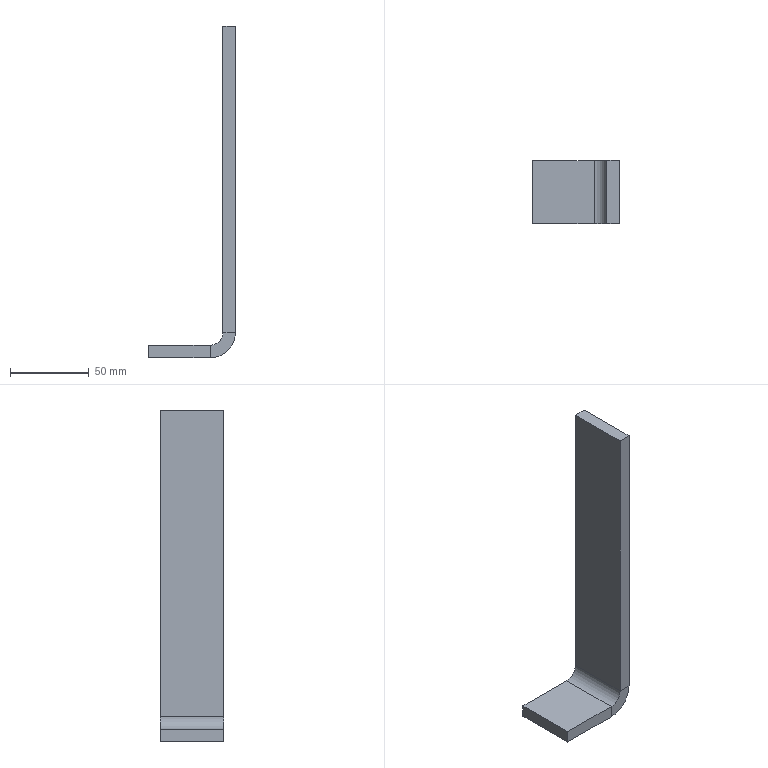Part | SolidWorks | features FlatPattern 1, SM3dBend 1, SMBaseFlange 1, SheetMetal 1 | 1 solid | 14 faces | box 55 x 40 x 210.02 mm | volume 80598 mm3 | plane 12 | cylinder 2 | commonest cylinder face diameters 16 x1 32 x1
STEP:
#1=CARTESIAN_POINT('',(-70.935,-20.,8.));
#2=VERTEX_POINT('',#1);
#3=CARTESIAN_POINT('',(-70.935,-20.,202.02));
#4=VERTEX_POINT('',#3);
#5=CARTESIAN_POINT('',(-70.935,-20.,-49.85));
#6=DIRECTION('',(0.,0.,1.));
#7=VECTOR('',#6,1000.);
#8=LINE('',#5,#7);
#9=EDGE_CURVE('',#2,#4,#8,.T.);
#10=ORIENTED_EDGE('',*,*,#9,.F.);
#11=CARTESIAN_POINT('',(-70.935,20.,8.));
#12=VERTEX_POINT('',#11);
#13=CARTESIAN_POINT('',(-70.935,0.,8.));
#14=DIRECTION('',(0.,1.,0.));
#15=VECTOR('',#14,1000.);
#16=LINE('',#13,#15);
#17=EDGE_CURVE('',#2,#12,#16,.T.);
#18=ORIENTED_EDGE('',*,*,#17,.T.);
#19=CARTESIAN_POINT('',(-70.935,20.,202.02));
#20=VERTEX_POINT('',#19);
#21=CARTESIAN_POINT('',(-70.935,20.,-49.85));
#22=DIRECTION('',(0.,0.,-1.));
#23=VECTOR('',#22,1000.);
#24=LINE('',#21,#23);
#25=EDGE_CURVE('',#20,#12,#24,.T.);
#26=ORIENTED_EDGE('',*,*,#25,.F.);
#27=CARTESIAN_POINT('',(-70.935,20.,202.02));
#28=DIRECTION('',(0.,1.,0.));
#29=VECTOR('',#28,1000.);
#30=LINE('',#27,#29);
#31=EDGE_CURVE('',#4,#20,#30,.T.);
#32=ORIENTED_EDGE('',*,*,#31,.F.);
#33=EDGE_LOOP('',(#10,#18,#26,#32));
#34=FACE_OUTER_BOUND('',#33,.T.);
#35=CARTESIAN_POINT('',(-70.935,0.,76.085));
#36=DIRECTION('',(-1.,0.,0.));
#37=DIRECTION('',(0.,0.,1.));
#38=AXIS2_PLACEMENT_3D('',#35,#36,#37);
#39=PLANE('',#38);
#40=ADVANCED_FACE('',(#34),#39,.F.);
#41=CARTESIAN_POINT('',(-78.935,-20.,202.02));
#42=VERTEX_POINT('',#41);
#43=CARTESIAN_POINT('',(-78.935,20.,202.02));
#44=VERTEX_POINT('',#43);
#45=CARTESIAN_POINT('',(-78.935,20.,202.02));
#46=DIRECTION('',(0.,1.,0.));
#47=VECTOR('',#46,1000.);
#48=LINE('',#45,#47);
#49=EDGE_CURVE('',#42,#44,#48,.T.);
#50=ORIENTED_EDGE('',*,*,#49,.F.);
#51=CARTESIAN_POINT('',(-70.935,-20.,202.02));
#52=DIRECTION('',(-1.,0.,0.));
#53=VECTOR('',#52,1000.);
#54=LINE('',#51,#53);
#55=EDGE_CURVE('',#4,#42,#54,.T.);
#56=ORIENTED_EDGE('',*,*,#55,.F.);
#57=ORIENTED_EDGE('',*,*,#31,.T.);
#58=CARTESIAN_POINT('',(-70.935,20.,202.02));
#59=DIRECTION('',(-1.,0.,0.));
#60=VECTOR('',#59,1000.);
#61=LINE('',#58,#60);
#62=EDGE_CURVE('',#20,#44,#61,.T.);
#63=ORIENTED_EDGE('',*,*,#62,.T.);
#64=EDGE_LOOP('',(#50,#56,#57,#63));
#65=FACE_OUTER_BOUND('',#64,.T.);
#66=CARTESIAN_POINT('',(-70.935,20.,202.02));
#67=DIRECTION('',(0.,0.,1.));
#68=DIRECTION('',(1.,0.,0.));
#69=AXIS2_PLACEMENT_3D('',#66,#67,#68);
#70=PLANE('',#69);
#71=ADVANCED_FACE('',(#65),#70,.T.);
#72=CARTESIAN_POINT('',(-78.935,-20.,8.));
#73=VERTEX_POINT('',#72);
#74=CARTESIAN_POINT('',(-70.935,-20.,8.));
#75=DIRECTION('',(-1.,0.,0.));
#76=VECTOR('',#75,1000.);
#77=LINE('',#74,#76);
#78=EDGE_CURVE('',#2,#73,#77,.T.);
#79=ORIENTED_EDGE('',*,*,#78,.F.);
#80=ORIENTED_EDGE('',*,*,#9,.T.);
#81=ORIENTED_EDGE('',*,*,#55,.T.);
#82=CARTESIAN_POINT('',(-78.935,-20.,-49.85));
#83=DIRECTION('',(0.,0.,1.));
#84=VECTOR('',#83,1000.);
#85=LINE('',#82,#84);
#86=EDGE_CURVE('',#73,#42,#85,.T.);
#87=ORIENTED_EDGE('',*,*,#86,.F.);
#88=EDGE_LOOP('',(#79,#80,#81,#87));
#89=FACE_OUTER_BOUND('',#88,.T.);
#90=CARTESIAN_POINT('',(-70.935,-20.,-49.85));
#91=DIRECTION('',(0.,-1.,0.));
#92=DIRECTION('',(1.,0.,0.));
#93=AXIS2_PLACEMENT_3D('',#90,#91,#92);
#94=PLANE('',#93);
#95=ADVANCED_FACE('',(#89),#94,.T.);
#96=CARTESIAN_POINT('',(-78.935,20.,8.));
#97=VERTEX_POINT('',#96);
#98=CARTESIAN_POINT('',(-70.935,20.,8.));
#99=DIRECTION('',(1.,0.,0.));
#100=VECTOR('',#99,1000.);
#101=LINE('',#98,#100);
#102=EDGE_CURVE('',#97,#12,#101,.T.);
#103=ORIENTED_EDGE('',*,*,#102,.F.);
#104=CARTESIAN_POINT('',(-78.935,20.,-49.85));
#105=DIRECTION('',(0.,0.,-1.));
#106=VECTOR('',#105,1000.);
#107=LINE('',#104,#106);
#108=EDGE_CURVE('',#44,#97,#107,.T.);
#109=ORIENTED_EDGE('',*,*,#108,.F.);
#110=ORIENTED_EDGE('',*,*,#62,.F.);
#111=ORIENTED_EDGE('',*,*,#25,.T.);
#112=EDGE_LOOP('',(#103,#109,#110,#111));
#113=FACE_OUTER_BOUND('',#112,.T.);
#114=CARTESIAN_POINT('',(-70.935,20.,-49.85));
#115=DIRECTION('',(0.,1.,0.));
#116=DIRECTION('',(-1.,0.,0.));
#117=AXIS2_PLACEMENT_3D('',#114,#115,#116);
#118=PLANE('',#117);
#119=ADVANCED_FACE('',(#113),#118,.T.);
#120=CARTESIAN_POINT('',(-78.935,0.,8.));
#121=DIRECTION('',(0.,1.,0.));
#122=VECTOR('',#121,1000.);
#123=LINE('',#120,#122);
#124=EDGE_CURVE('',#73,#97,#123,.T.);
#125=ORIENTED_EDGE('',*,*,#124,.F.);
#126=ORIENTED_EDGE('',*,*,#86,.T.);
#127=ORIENTED_EDGE('',*,*,#49,.T.);
#128=ORIENTED_EDGE('',*,*,#108,.T.);
#129=EDGE_LOOP('',(#125,#126,#127,#128));
#130=FACE_OUTER_BOUND('',#129,.T.);
#131=CARTESIAN_POINT('',(-78.935,0.,76.085));
#132=DIRECTION('',(-1.,0.,0.));
#133=DIRECTION('',(0.,0.,1.));
#134=AXIS2_PLACEMENT_3D('',#131,#132,#133);
#135=PLANE('',#134);
#136=ADVANCED_FACE('',(#130),#135,.T.);
#137=CARTESIAN_POINT('',(-125.935,20.,0.));
#138=VERTEX_POINT('',#137);
#139=CARTESIAN_POINT('',(-125.935,-20.,0.));
#140=VERTEX_POINT('',#139);
#141=CARTESIAN_POINT('',(-125.935,20.,0.));
#142=DIRECTION('',(0.,-1.,0.));
#143=VECTOR('',#142,1000.);
#144=LINE('',#141,#143);
#145=EDGE_CURVE('',#138,#140,#144,.T.);
#146=ORIENTED_EDGE('',*,*,#145,.F.);
#147=CARTESIAN_POINT('',(-125.935,20.,-8.));
#148=VERTEX_POINT('',#147);
#149=CARTESIAN_POINT('',(-125.935,20.,-8.));
#150=DIRECTION('',(0.,0.,1.));
#151=VECTOR('',#150,1000.);
#152=LINE('',#149,#151);
#153=EDGE_CURVE('',#148,#138,#152,.T.);
#154=ORIENTED_EDGE('',*,*,#153,.F.);
#155=CARTESIAN_POINT('',(-125.935,-20.,-8.));
#156=VERTEX_POINT('',#155);
#157=CARTESIAN_POINT('',(-125.935,20.,-8.));
#158=DIRECTION('',(0.,-1.,0.));
#159=VECTOR('',#158,1000.);
#160=LINE('',#157,#159);
#161=EDGE_CURVE('',#148,#156,#160,.T.);
#162=ORIENTED_EDGE('',*,*,#161,.T.);
#163=CARTESIAN_POINT('',(-125.935,-20.,-8.));
#164=DIRECTION('',(0.,0.,1.));
#165=VECTOR('',#164,1000.);
#166=LINE('',#163,#165);
#167=EDGE_CURVE('',#156,#140,#166,.T.);
#168=ORIENTED_EDGE('',*,*,#167,.T.);
#169=EDGE_LOOP('',(#146,#154,#162,#168));
#170=FACE_OUTER_BOUND('',#169,.T.);
#171=CARTESIAN_POINT('',(-125.935,20.,-8.));
#172=DIRECTION('',(-1.,0.,0.));
#173=DIRECTION('',(0.,0.,1.));
#174=AXIS2_PLACEMENT_3D('',#171,#172,#173);
#175=PLANE('',#174);
#176=ADVANCED_FACE('',(#170),#175,.T.);
#177=CARTESIAN_POINT('',(-86.935,-20.,-8.));
#178=VERTEX_POINT('',#177);
#179=CARTESIAN_POINT('',(-86.935,20.,-8.));
#180=VERTEX_POINT('',#179);
#181=CARTESIAN_POINT('',(-86.935,0.,-8.));
#182=DIRECTION('',(0.,1.,0.));
#183=VECTOR('',#182,1000.);
#184=LINE('',#181,#183);
#185=EDGE_CURVE('',#178,#180,#184,.T.);
#186=ORIENTED_EDGE('',*,*,#185,.F.);
#187=CARTESIAN_POINT('',(-125.935,-20.,-8.));
#188=DIRECTION('',(1.,0.,0.));
#189=VECTOR('',#188,1000.);
#190=LINE('',#187,#189);
#191=EDGE_CURVE('',#156,#178,#190,.T.);
#192=ORIENTED_EDGE('',*,*,#191,.F.);
#193=ORIENTED_EDGE('',*,*,#161,.F.);
#194=CARTESIAN_POINT('',(-125.935,20.,-8.));
#195=DIRECTION('',(-1.,0.,0.));
#196=VECTOR('',#195,1000.);
#197=LINE('',#194,#196);
#198=EDGE_CURVE('',#180,#148,#197,.T.);
#199=ORIENTED_EDGE('',*,*,#198,.F.);
#200=EDGE_LOOP('',(#186,#192,#193,#199));
#201=FACE_OUTER_BOUND('',#200,.T.);
#202=CARTESIAN_POINT('',(0.,0.,-8.));
#203=DIRECTION('',(0.,0.,1.));
#204=DIRECTION('',(1.,0.,0.));
#205=AXIS2_PLACEMENT_3D('',#202,#203,#204);
#206=PLANE('',#205);
#207=ADVANCED_FACE('',(#201),#206,.F.);
#208=ORIENTED_EDGE('',*,*,#191,.T.);
#209=CARTESIAN_POINT('',(-86.935,-20.,0.));
#210=VERTEX_POINT('',#209);
#211=CARTESIAN_POINT('',(-86.935,-20.,-8.));
#212=DIRECTION('',(0.,0.,1.));
#213=VECTOR('',#212,1000.);
#214=LINE('',#211,#213);
#215=EDGE_CURVE('',#178,#210,#214,.T.);
#216=ORIENTED_EDGE('',*,*,#215,.T.);
#217=CARTESIAN_POINT('',(-125.935,-20.,0.));
#218=DIRECTION('',(1.,0.,0.));
#219=VECTOR('',#218,1000.);
#220=LINE('',#217,#219);
#221=EDGE_CURVE('',#140,#210,#220,.T.);
#222=ORIENTED_EDGE('',*,*,#221,.F.);
#223=ORIENTED_EDGE('',*,*,#167,.F.);
#224=EDGE_LOOP('',(#208,#216,#222,#223));
#225=FACE_OUTER_BOUND('',#224,.T.);
#226=CARTESIAN_POINT('',(-125.935,-20.,-8.));
#227=DIRECTION('',(0.,-1.,0.));
#228=DIRECTION('',(0.,0.,-1.));
#229=AXIS2_PLACEMENT_3D('',#226,#227,#228);
#230=PLANE('',#229);
#231=ADVANCED_FACE('',(#225),#230,.T.);
#232=ORIENTED_EDGE('',*,*,#221,.T.);
#233=CARTESIAN_POINT('',(-86.935,20.,0.));
#234=VERTEX_POINT('',#233);
#235=CARTESIAN_POINT('',(-86.935,0.,0.));
#236=DIRECTION('',(0.,1.,0.));
#237=VECTOR('',#236,1000.);
#238=LINE('',#235,#237);
#239=EDGE_CURVE('',#210,#234,#238,.T.);
#240=ORIENTED_EDGE('',*,*,#239,.T.);
#241=CARTESIAN_POINT('',(-125.935,20.,0.));
#242=DIRECTION('',(-1.,0.,0.));
#243=VECTOR('',#242,1000.);
#244=LINE('',#241,#243);
#245=EDGE_CURVE('',#234,#138,#244,.T.);
#246=ORIENTED_EDGE('',*,*,#245,.T.);
#247=ORIENTED_EDGE('',*,*,#145,.T.);
#248=EDGE_LOOP('',(#232,#240,#246,#247));
#249=FACE_OUTER_BOUND('',#248,.T.);
#250=CARTESIAN_POINT('',(0.,0.,0.));
#251=DIRECTION('',(0.,0.,1.));
#252=DIRECTION('',(1.,0.,0.));
#253=AXIS2_PLACEMENT_3D('',#250,#251,#252);
#254=PLANE('',#253);
#255=ADVANCED_FACE('',(#249),#254,.T.);
#256=ORIENTED_EDGE('',*,*,#245,.F.);
#257=CARTESIAN_POINT('',(-86.935,20.,-8.));
#258=DIRECTION('',(0.,0.,-1.));
#259=VECTOR('',#258,1000.);
#260=LINE('',#257,#259);
#261=EDGE_CURVE('',#234,#180,#260,.T.);
#262=ORIENTED_EDGE('',*,*,#261,.T.);
#263=ORIENTED_EDGE('',*,*,#198,.T.);
#264=ORIENTED_EDGE('',*,*,#153,.T.);
#265=EDGE_LOOP('',(#256,#262,#263,#264));
#266=FACE_OUTER_BOUND('',#265,.T.);
#267=CARTESIAN_POINT('',(-125.935,20.,-8.));
#268=DIRECTION('',(0.,1.,0.));
#269=DIRECTION('',(0.,0.,1.));
#270=AXIS2_PLACEMENT_3D('',#267,#268,#269);
#271=PLANE('',#270);
#272=ADVANCED_FACE('',(#266),#271,.T.);
#273=ORIENTED_EDGE('',*,*,#78,.T.);
#274=CARTESIAN_POINT('',(-86.935,-20.,8.));
#275=DIRECTION('',(0.,1.,0.));
#276=DIRECTION('',(0.,0.,-1.));
#277=AXIS2_PLACEMENT_3D('',#274,#275,#276);
#278=CIRCLE('',#277,8.);
#279=EDGE_CURVE('',#73,#210,#278,.T.);
#280=ORIENTED_EDGE('',*,*,#279,.T.);
#281=ORIENTED_EDGE('',*,*,#215,.F.);
#282=CARTESIAN_POINT('',(-86.935,-20.,8.));
#283=DIRECTION('',(0.,1.,0.));
#284=DIRECTION('',(0.,0.,-1.));
#285=AXIS2_PLACEMENT_3D('',#282,#283,#284);
#286=CIRCLE('',#285,16.);
#287=EDGE_CURVE('',#2,#178,#286,.T.);
#288=ORIENTED_EDGE('',*,*,#287,.F.);
#289=EDGE_LOOP('',(#273,#280,#281,#288));
#290=FACE_OUTER_BOUND('',#289,.T.);
#291=CARTESIAN_POINT('',(-86.935,-20.,8.));
#292=DIRECTION('',(0.,-1.,0.));
#293=DIRECTION('',(0.,0.,-1.));
#294=AXIS2_PLACEMENT_3D('',#291,#292,#293);
#295=PLANE('',#294);
#296=ADVANCED_FACE('',(#290),#295,.T.);
#297=CARTESIAN_POINT('',(-86.935,20.,8.));
#298=DIRECTION('',(0.,-1.,0.));
#299=DIRECTION('',(0.,0.,-1.));
#300=AXIS2_PLACEMENT_3D('',#297,#298,#299);
#301=CIRCLE('',#300,8.);
#302=EDGE_CURVE('',#234,#97,#301,.T.);
#303=ORIENTED_EDGE('',*,*,#302,.T.);
#304=ORIENTED_EDGE('',*,*,#102,.T.);
#305=CARTESIAN_POINT('',(-86.935,20.,8.));
#306=DIRECTION('',(0.,-1.,0.));
#307=DIRECTION('',(0.,0.,1.));
#308=AXIS2_PLACEMENT_3D('',#305,#306,#307);
#309=CIRCLE('',#308,16.);
#310=EDGE_CURVE('',#180,#12,#309,.T.);
#311=ORIENTED_EDGE('',*,*,#310,.F.);
#312=ORIENTED_EDGE('',*,*,#261,.F.);
#313=EDGE_LOOP('',(#303,#304,#311,#312));
#314=FACE_OUTER_BOUND('',#313,.T.);
#315=CARTESIAN_POINT('',(-86.935,20.,8.));
#316=DIRECTION('',(0.,1.,0.));
#317=DIRECTION('',(0.,0.,1.));
#318=AXIS2_PLACEMENT_3D('',#315,#316,#317);
#319=PLANE('',#318);
#320=ADVANCED_FACE('',(#314),#319,.T.);
#321=ORIENTED_EDGE('',*,*,#185,.T.);
#322=ORIENTED_EDGE('',*,*,#310,.T.);
#323=ORIENTED_EDGE('',*,*,#17,.F.);
#324=ORIENTED_EDGE('',*,*,#287,.T.);
#325=EDGE_LOOP('',(#321,#322,#323,#324));
#326=FACE_OUTER_BOUND('',#325,.T.);
#327=CARTESIAN_POINT('',(-86.935,44.937,8.));
#328=DIRECTION('',(0.,-1.,0.));
#329=DIRECTION('',(0.,0.,-1.));
#330=AXIS2_PLACEMENT_3D('',#327,#328,#329);
#331=CYLINDRICAL_SURFACE('',#330,16.);
#332=ADVANCED_FACE('',(#326),#331,.T.);
#333=ORIENTED_EDGE('',*,*,#239,.F.);
#334=ORIENTED_EDGE('',*,*,#279,.F.);
#335=ORIENTED_EDGE('',*,*,#124,.T.);
#336=ORIENTED_EDGE('',*,*,#302,.F.);
#337=EDGE_LOOP('',(#333,#334,#335,#336));
#338=FACE_OUTER_BOUND('',#337,.T.);
#339=CARTESIAN_POINT('',(-86.935,44.937,8.));
#340=DIRECTION('',(0.,-1.,0.));
#341=DIRECTION('',(0.,0.,-1.));
#342=AXIS2_PLACEMENT_3D('',#339,#340,#341);
#343=CYLINDRICAL_SURFACE('',#342,8.);
#344=ADVANCED_FACE('',(#338),#343,.F.);
#345=CLOSED_SHELL('',(#40,#71,#95,#119,#136,#176,#207,#231,#255,#272,#296,#320,#332,#344));
#346=MANIFOLD_SOLID_BREP('',#345);
#347=CARTESIAN_POINT('',(0.,0.,0.));
#348=DIRECTION('',(0.,0.,1.));
#349=DIRECTION('',(1.,0.,0.));
#350=AXIS2_PLACEMENT_3D('',#347,#348,#349);
#351=(LENGTH_UNIT()NAMED_UNIT(*)SI_UNIT(.MILLI.,.METRE.));
#352=UNCERTAINTY_MEASURE_WITH_UNIT(LENGTH_MEASURE(0.00001),#351,'','');
#353=(NAMED_UNIT(*)PLANE_ANGLE_UNIT()SI_UNIT($,.RADIAN.));
#354=(NAMED_UNIT(*)SI_UNIT($,.STERADIAN.)SOLID_ANGLE_UNIT());
#355=(GEOMETRIC_REPRESENTATION_CONTEXT(3)GLOBAL_UNCERTAINTY_ASSIGNED_CONTEXT((#352))GLOBAL_UNIT_ASSIGNED_CONTEXT((#351,#353,#354))REPRESENTATION_CONTEXT('',''));
#356=ADVANCED_BREP_SHAPE_REPRESENTATION('',(#346,#350),#355);